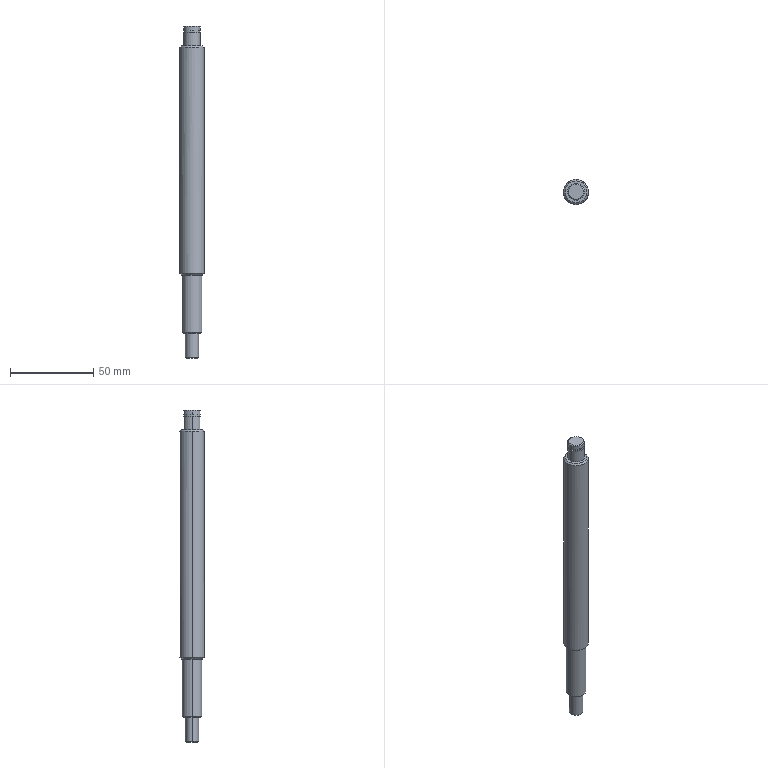Part | STEP file | HI_LCP02-16-16-L200-F15-P8 | 1 solid | 29 faces | box 15 x 15 x 200 mm | volume 29982 mm3 | cylinder 12 | cone 10 | plane 7 | commonest cylinder face diameters 10 x4 8 x2 9.6 x2 12 x2 15 x2